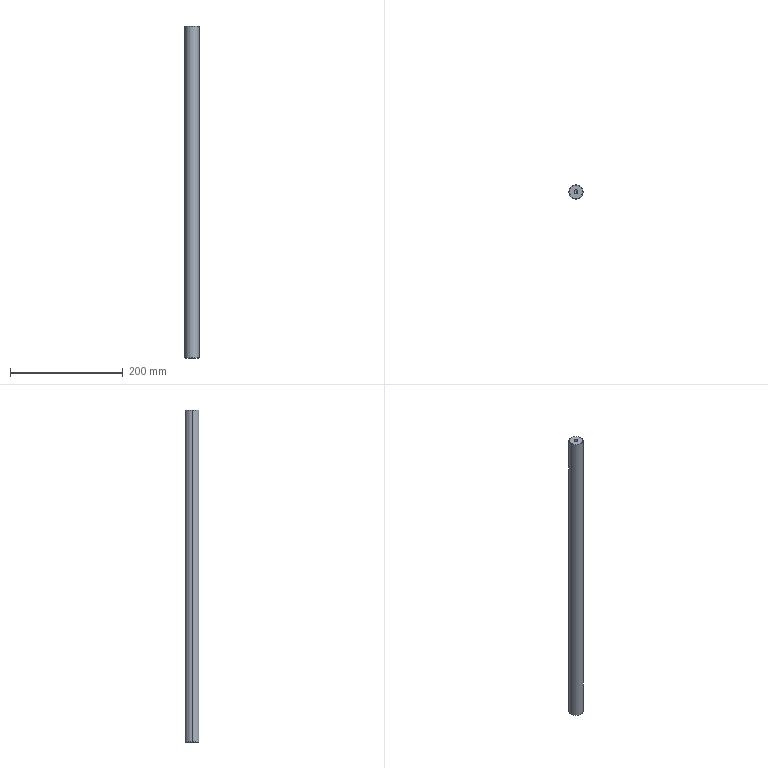Part | SolidWorks | features HoleWzd 2, Chamfer 1, Extrusion 1 | 1 solid | 18 faces | box 25 x 25 x 590 mm | volume 288109 mm3 | cone 10 | cylinder 6 | plane 2 | commonest cylinder face diameters 6.8 x4 25 x2
STEP:
#1=CARTESIAN_POINT('',(12.,0.,590.));
#2=VERTEX_POINT('',#1);
#3=CARTESIAN_POINT('',(-12.,0.,590.));
#4=VERTEX_POINT('',#3);
#5=CARTESIAN_POINT('',(0.,0.,590.));
#6=DIRECTION('',(0.,0.,1.));
#7=DIRECTION('',(1.,0.,0.));
#8=AXIS2_PLACEMENT_3D('',#5,#6,#7);
#9=CIRCLE('',#8,12.);
#10=EDGE_CURVE('',#2,#4,#9,.T.);
#11=ORIENTED_EDGE('',*,*,#10,.F.);
#12=CARTESIAN_POINT('',(12.5,0.,589.5));
#13=VERTEX_POINT('',#12);
#14=CARTESIAN_POINT('',(12.,0.,590.));
#15=DIRECTION('',(0.7071,0.,-0.7071));
#16=VECTOR('',#15,1000.);
#17=LINE('',#14,#16);
#18=EDGE_CURVE('',#2,#13,#17,.T.);
#19=ORIENTED_EDGE('',*,*,#18,.T.);
#20=CARTESIAN_POINT('',(-12.5,0.,589.5));
#21=VERTEX_POINT('',#20);
#22=CARTESIAN_POINT('',(0.,0.,589.5));
#23=DIRECTION('',(0.,0.,-1.));
#24=DIRECTION('',(1.,0.,0.));
#25=AXIS2_PLACEMENT_3D('',#22,#23,#24);
#26=CIRCLE('',#25,12.5);
#27=EDGE_CURVE('',#21,#13,#26,.T.);
#28=ORIENTED_EDGE('',*,*,#27,.F.);
#29=CARTESIAN_POINT('',(-12.,0.,590.));
#30=DIRECTION('',(-0.7071,0.,-0.7071));
#31=VECTOR('',#30,1000.);
#32=LINE('',#29,#31);
#33=EDGE_CURVE('',#4,#21,#32,.T.);
#34=ORIENTED_EDGE('',*,*,#33,.F.);
#35=EDGE_LOOP('',(#11,#19,#28,#34));
#36=FACE_OUTER_BOUND('',#35,.T.);
#37=CARTESIAN_POINT('',(0.,0.,590.));
#38=DIRECTION('',(0.,0.,-1.));
#39=DIRECTION('',(-1.,0.,0.));
#40=AXIS2_PLACEMENT_3D('',#37,#38,#39);
#41=CONICAL_SURFACE('',#40,12.,0.7854);
#42=ADVANCED_FACE('',(#36),#41,.T.);
#43=CARTESIAN_POINT('',(3.4,0.,0.5));
#44=VERTEX_POINT('',#43);
#45=CARTESIAN_POINT('',(-3.4,0.,0.5));
#46=VERTEX_POINT('',#45);
#47=CARTESIAN_POINT('',(0.,0.,0.5));
#48=DIRECTION('',(0.,0.,-1.));
#49=DIRECTION('',(1.,0.,0.));
#50=AXIS2_PLACEMENT_3D('',#47,#48,#49);
#51=CIRCLE('',#50,3.4);
#52=EDGE_CURVE('',#44,#46,#51,.T.);
#53=ORIENTED_EDGE('',*,*,#52,.F.);
#54=CARTESIAN_POINT('',(3.9,0.,0.));
#55=VERTEX_POINT('',#54);
#56=CARTESIAN_POINT('',(3.4,0.,0.5));
#57=DIRECTION('',(0.7071,0.,-0.7071));
#58=VECTOR('',#57,1000.);
#59=LINE('',#56,#58);
#60=EDGE_CURVE('',#44,#55,#59,.T.);
#61=ORIENTED_EDGE('',*,*,#60,.T.);
#62=CARTESIAN_POINT('',(-3.9,0.,0.));
#63=VERTEX_POINT('',#62);
#64=CARTESIAN_POINT('',(0.,0.,0.));
#65=DIRECTION('',(0.,0.,1.));
#66=DIRECTION('',(1.,0.,0.));
#67=AXIS2_PLACEMENT_3D('',#64,#65,#66);
#68=CIRCLE('',#67,3.9);
#69=EDGE_CURVE('',#63,#55,#68,.T.);
#70=ORIENTED_EDGE('',*,*,#69,.F.);
#71=CARTESIAN_POINT('',(-3.4,0.,0.5));
#72=DIRECTION('',(-0.7071,0.,-0.7071));
#73=VECTOR('',#72,1000.);
#74=LINE('',#71,#73);
#75=EDGE_CURVE('',#46,#63,#74,.T.);
#76=ORIENTED_EDGE('',*,*,#75,.F.);
#77=EDGE_LOOP('',(#53,#61,#70,#76));
#78=FACE_OUTER_BOUND('',#77,.T.);
#79=CARTESIAN_POINT('',(0.,0.,0.5));
#80=DIRECTION('',(0.,0.,-1.));
#81=DIRECTION('',(-1.,0.,0.));
#82=AXIS2_PLACEMENT_3D('',#79,#80,#81);
#83=CONICAL_SURFACE('',#82,3.4,0.7854);
#84=ADVANCED_FACE('',(#78),#83,.F.);
#85=CARTESIAN_POINT('',(-12.,0.,0.));
#86=VERTEX_POINT('',#85);
#87=CARTESIAN_POINT('',(12.,0.,0.));
#88=VERTEX_POINT('',#87);
#89=CARTESIAN_POINT('',(0.,0.,0.));
#90=DIRECTION('',(0.,0.,-1.));
#91=DIRECTION('',(1.,0.,0.));
#92=AXIS2_PLACEMENT_3D('',#89,#90,#91);
#93=CIRCLE('',#92,12.);
#94=EDGE_CURVE('',#86,#88,#93,.T.);
#95=ORIENTED_EDGE('',*,*,#94,.F.);
#96=CARTESIAN_POINT('',(-12.5,0.,0.5));
#97=VERTEX_POINT('',#96);
#98=CARTESIAN_POINT('',(-12.5,0.,0.5));
#99=DIRECTION('',(-0.7071,0.,0.7071));
#100=VECTOR('',#99,1000.);
#101=LINE('',#98,#100);
#102=EDGE_CURVE('',#86,#97,#101,.T.);
#103=ORIENTED_EDGE('',*,*,#102,.T.);
#104=CARTESIAN_POINT('',(12.5,0.,0.5));
#105=VERTEX_POINT('',#104);
#106=CARTESIAN_POINT('',(0.,0.,0.5));
#107=DIRECTION('',(0.,0.,1.));
#108=DIRECTION('',(1.,0.,0.));
#109=AXIS2_PLACEMENT_3D('',#106,#107,#108);
#110=CIRCLE('',#109,12.5);
#111=EDGE_CURVE('',#105,#97,#110,.T.);
#112=ORIENTED_EDGE('',*,*,#111,.F.);
#113=CARTESIAN_POINT('',(12.5,0.,0.5));
#114=DIRECTION('',(0.7071,0.,0.7071));
#115=VECTOR('',#114,1000.);
#116=LINE('',#113,#115);
#117=EDGE_CURVE('',#88,#105,#116,.T.);
#118=ORIENTED_EDGE('',*,*,#117,.F.);
#119=EDGE_LOOP('',(#95,#103,#112,#118));
#120=FACE_OUTER_BOUND('',#119,.T.);
#121=CARTESIAN_POINT('',(0.,0.,0.5));
#122=DIRECTION('',(0.,0.,1.));
#123=DIRECTION('',(1.,0.,0.));
#124=AXIS2_PLACEMENT_3D('',#121,#122,#123);
#125=CONICAL_SURFACE('',#124,12.5,0.7854);
#126=ADVANCED_FACE('',(#120),#125,.T.);
#127=CARTESIAN_POINT('',(3.4,0.,19.75));
#128=VERTEX_POINT('',#127);
#129=CARTESIAN_POINT('',(-3.4,0.,19.75));
#130=VERTEX_POINT('',#129);
#131=CARTESIAN_POINT('',(0.,0.,19.75));
#132=DIRECTION('',(0.,0.,-1.));
#133=DIRECTION('',(-1.,0.,0.));
#134=AXIS2_PLACEMENT_3D('',#131,#132,#133);
#135=CIRCLE('',#134,3.4);
#136=EDGE_CURVE('',#128,#130,#135,.T.);
#137=ORIENTED_EDGE('',*,*,#136,.F.);
#138=CARTESIAN_POINT('',(3.4,0.,0.));
#139=DIRECTION('',(0.,0.,-1.));
#140=VECTOR('',#139,1000.);
#141=LINE('',#138,#140);
#142=EDGE_CURVE('',#128,#44,#141,.T.);
#143=ORIENTED_EDGE('',*,*,#142,.T.);
#144=ORIENTED_EDGE('',*,*,#52,.T.);
#145=CARTESIAN_POINT('',(-3.4,0.,0.));
#146=DIRECTION('',(0.,0.,-1.));
#147=VECTOR('',#146,1000.);
#148=LINE('',#145,#147);
#149=EDGE_CURVE('',#130,#46,#148,.T.);
#150=ORIENTED_EDGE('',*,*,#149,.F.);
#151=EDGE_LOOP('',(#137,#143,#144,#150));
#152=FACE_OUTER_BOUND('',#151,.T.);
#153=CARTESIAN_POINT('',(0.,0.,0.));
#154=DIRECTION('',(0.,0.,-1.));
#155=DIRECTION('',(-1.,0.,0.));
#156=AXIS2_PLACEMENT_3D('',#153,#154,#155);
#157=CYLINDRICAL_SURFACE('',#156,3.4);
#158=ADVANCED_FACE('',(#152),#157,.F.);
#159=CARTESIAN_POINT('',(0.,0.,21.793));
#160=VERTEX_POINT('',#159);
#161=CARTESIAN_POINT('',(-3.4,0.,19.75));
#162=DIRECTION('',(-0.8572,0.,-0.515));
#163=VECTOR('',#162,1000.);
#164=LINE('',#161,#163);
#165=EDGE_CURVE('',#160,#130,#164,.T.);
#166=ORIENTED_EDGE('',*,*,#165,.F.);
#167=CARTESIAN_POINT('',(3.4,0.,19.75));
#168=DIRECTION('',(0.8572,0.,-0.515));
#169=VECTOR('',#168,1000.);
#170=LINE('',#167,#169);
#171=EDGE_CURVE('',#160,#128,#170,.T.);
#172=ORIENTED_EDGE('',*,*,#171,.T.);
#173=ORIENTED_EDGE('',*,*,#136,.T.);
#174=EDGE_LOOP('',(#166,#172,#173));
#175=FACE_OUTER_BOUND('',#174,.T.);
#176=CARTESIAN_POINT('',(0.,0.,19.75));
#177=DIRECTION('',(0.,0.,-1.));
#178=DIRECTION('',(-1.,0.,0.));
#179=AXIS2_PLACEMENT_3D('',#176,#177,#178);
#180=CONICAL_SURFACE('',#179,3.4,1.03);
#181=ADVANCED_FACE('',(#175),#180,.F.);
#182=CARTESIAN_POINT('',(-3.4,0.,570.25));
#183=VERTEX_POINT('',#182);
#184=CARTESIAN_POINT('',(3.4,0.,570.25));
#185=VERTEX_POINT('',#184);
#186=CARTESIAN_POINT('',(0.,0.,570.25));
#187=DIRECTION('',(0.,0.,1.));
#188=DIRECTION('',(1.,0.,0.));
#189=AXIS2_PLACEMENT_3D('',#186,#187,#188);
#190=CIRCLE('',#189,3.4);
#191=EDGE_CURVE('',#183,#185,#190,.T.);
#192=ORIENTED_EDGE('',*,*,#191,.F.);
#193=CARTESIAN_POINT('',(-3.4,0.,590.));
#194=VERTEX_POINT('',#193);
#195=CARTESIAN_POINT('',(-3.4,0.,590.));
#196=DIRECTION('',(0.,0.,1.));
#197=VECTOR('',#196,1000.);
#198=LINE('',#195,#197);
#199=EDGE_CURVE('',#183,#194,#198,.T.);
#200=ORIENTED_EDGE('',*,*,#199,.T.);
#201=CARTESIAN_POINT('',(3.4,0.,590.));
#202=VERTEX_POINT('',#201);
#203=CARTESIAN_POINT('',(0.,0.,590.));
#204=DIRECTION('',(0.,0.,1.));
#205=DIRECTION('',(1.,0.,0.));
#206=AXIS2_PLACEMENT_3D('',#203,#204,#205);
#207=CIRCLE('',#206,3.4);
#208=EDGE_CURVE('',#194,#202,#207,.T.);
#209=ORIENTED_EDGE('',*,*,#208,.T.);
#210=CARTESIAN_POINT('',(3.4,0.,590.));
#211=DIRECTION('',(0.,0.,1.));
#212=VECTOR('',#211,1000.);
#213=LINE('',#210,#212);
#214=EDGE_CURVE('',#185,#202,#213,.T.);
#215=ORIENTED_EDGE('',*,*,#214,.F.);
#216=EDGE_LOOP('',(#192,#200,#209,#215));
#217=FACE_OUTER_BOUND('',#216,.T.);
#218=CARTESIAN_POINT('',(0.,0.,590.));
#219=DIRECTION('',(0.,0.,1.));
#220=DIRECTION('',(1.,0.,0.));
#221=AXIS2_PLACEMENT_3D('',#218,#219,#220);
#222=CYLINDRICAL_SURFACE('',#221,3.4);
#223=ADVANCED_FACE('',(#217),#222,.F.);
#224=CARTESIAN_POINT('',(0.,0.,568.207));
#225=VERTEX_POINT('',#224);
#226=CARTESIAN_POINT('',(3.4,0.,570.25));
#227=DIRECTION('',(0.8572,0.,0.515));
#228=VECTOR('',#227,1000.);
#229=LINE('',#226,#228);
#230=EDGE_CURVE('',#225,#185,#229,.T.);
#231=ORIENTED_EDGE('',*,*,#230,.F.);
#232=CARTESIAN_POINT('',(-3.4,0.,570.25));
#233=DIRECTION('',(-0.8572,0.,0.515));
#234=VECTOR('',#233,1000.);
#235=LINE('',#232,#234);
#236=EDGE_CURVE('',#225,#183,#235,.T.);
#237=ORIENTED_EDGE('',*,*,#236,.T.);
#238=ORIENTED_EDGE('',*,*,#191,.T.);
#239=EDGE_LOOP('',(#231,#237,#238));
#240=FACE_OUTER_BOUND('',#239,.T.);
#241=CARTESIAN_POINT('',(0.,0.,570.25));
#242=DIRECTION('',(0.,0.,1.));
#243=DIRECTION('',(1.,0.,0.));
#244=AXIS2_PLACEMENT_3D('',#241,#242,#243);
#245=CONICAL_SURFACE('',#244,3.4,1.03);
#246=ADVANCED_FACE('',(#240),#245,.F.);
#247=ORIENTED_EDGE('',*,*,#27,.T.);
#248=CARTESIAN_POINT('',(12.5,0.,590.));
#249=DIRECTION('',(0.,0.,-1.));
#250=VECTOR('',#249,1000.);
#251=LINE('',#248,#250);
#252=EDGE_CURVE('',#13,#105,#251,.T.);
#253=ORIENTED_EDGE('',*,*,#252,.T.);
#254=ORIENTED_EDGE('',*,*,#111,.T.);
#255=CARTESIAN_POINT('',(-12.5,0.,590.));
#256=DIRECTION('',(0.,0.,-1.));
#257=VECTOR('',#256,1000.);
#258=LINE('',#255,#257);
#259=EDGE_CURVE('',#21,#97,#258,.T.);
#260=ORIENTED_EDGE('',*,*,#259,.F.);
#261=EDGE_LOOP('',(#247,#253,#254,#260));
#262=FACE_OUTER_BOUND('',#261,.T.);
#263=CARTESIAN_POINT('',(0.,0.,590.));
#264=DIRECTION('',(0.,0.,-1.));
#265=DIRECTION('',(-1.,0.,0.));
#266=AXIS2_PLACEMENT_3D('',#263,#264,#265);
#267=CYLINDRICAL_SURFACE('',#266,12.5);
#268=ADVANCED_FACE('',(#262),#267,.T.);
#269=ORIENTED_EDGE('',*,*,#252,.F.);
#270=CARTESIAN_POINT('',(0.,0.,589.5));
#271=DIRECTION('',(0.,0.,-1.));
#272=DIRECTION('',(1.,0.,0.));
#273=AXIS2_PLACEMENT_3D('',#270,#271,#272);
#274=CIRCLE('',#273,12.5);
#275=EDGE_CURVE('',#13,#21,#274,.T.);
#276=ORIENTED_EDGE('',*,*,#275,.T.);
#277=ORIENTED_EDGE('',*,*,#259,.T.);
#278=CARTESIAN_POINT('',(0.,0.,0.5));
#279=DIRECTION('',(0.,0.,1.));
#280=DIRECTION('',(1.,0.,0.));
#281=AXIS2_PLACEMENT_3D('',#278,#279,#280);
#282=CIRCLE('',#281,12.5);
#283=EDGE_CURVE('',#97,#105,#282,.T.);
#284=ORIENTED_EDGE('',*,*,#283,.T.);
#285=EDGE_LOOP('',(#269,#276,#277,#284));
#286=FACE_OUTER_BOUND('',#285,.T.);
#287=CARTESIAN_POINT('',(0.,0.,590.));
#288=DIRECTION('',(0.,0.,-1.));
#289=DIRECTION('',(-1.,0.,0.));
#290=AXIS2_PLACEMENT_3D('',#287,#288,#289);
#291=CYLINDRICAL_SURFACE('',#290,12.5);
#292=ADVANCED_FACE('',(#286),#291,.T.);
#293=CARTESIAN_POINT('',(0.,0.,590.));
#294=DIRECTION('',(0.,0.,1.));
#295=DIRECTION('',(1.,0.,0.));
#296=AXIS2_PLACEMENT_3D('',#293,#294,#295);
#297=CIRCLE('',#296,12.);
#298=EDGE_CURVE('',#4,#2,#297,.T.);
#299=ORIENTED_EDGE('',*,*,#298,.T.);
#300=ORIENTED_EDGE('',*,*,#10,.T.);
#301=EDGE_LOOP('',(#299,#300));
#302=FACE_OUTER_BOUND('',#301,.T.);
#303=CARTESIAN_POINT('',(0.,0.,590.));
#304=DIRECTION('',(0.,0.,1.));
#305=DIRECTION('',(1.,0.,0.));
#306=AXIS2_PLACEMENT_3D('',#303,#304,#305);
#307=CIRCLE('',#306,3.4);
#308=EDGE_CURVE('',#202,#194,#307,.T.);
#309=ORIENTED_EDGE('',*,*,#308,.F.);
#310=ORIENTED_EDGE('',*,*,#208,.F.);
#311=EDGE_LOOP('',(#309,#310));
#312=FACE_BOUND('',#311,.T.);
#313=CARTESIAN_POINT('',(0.,0.,590.));
#314=DIRECTION('',(0.,0.,1.));
#315=DIRECTION('',(1.,0.,0.));
#316=AXIS2_PLACEMENT_3D('',#313,#314,#315);
#317=PLANE('',#316);
#318=ADVANCED_FACE('',(#302,#312),#317,.T.);
#319=CARTESIAN_POINT('',(0.,0.,0.));
#320=DIRECTION('',(0.,0.,-1.));
#321=DIRECTION('',(1.,0.,0.));
#322=AXIS2_PLACEMENT_3D('',#319,#320,#321);
#323=CIRCLE('',#322,12.);
#324=EDGE_CURVE('',#88,#86,#323,.T.);
#325=ORIENTED_EDGE('',*,*,#324,.T.);
#326=ORIENTED_EDGE('',*,*,#94,.T.);
#327=EDGE_LOOP('',(#325,#326));
#328=FACE_OUTER_BOUND('',#327,.T.);
#329=ORIENTED_EDGE('',*,*,#69,.T.);
#330=CARTESIAN_POINT('',(0.,0.,0.));
#331=DIRECTION('',(0.,0.,1.));
#332=DIRECTION('',(1.,0.,0.));
#333=AXIS2_PLACEMENT_3D('',#330,#331,#332);
#334=CIRCLE('',#333,3.9);
#335=EDGE_CURVE('',#55,#63,#334,.T.);
#336=ORIENTED_EDGE('',*,*,#335,.T.);
#337=EDGE_LOOP('',(#329,#336));
#338=FACE_BOUND('',#337,.T.);
#339=CARTESIAN_POINT('',(0.,0.,0.));
#340=DIRECTION('',(0.,0.,1.));
#341=DIRECTION('',(1.,0.,0.));
#342=AXIS2_PLACEMENT_3D('',#339,#340,#341);
#343=PLANE('',#342);
#344=ADVANCED_FACE('',(#328,#338),#343,.F.);
#345=ORIENTED_EDGE('',*,*,#236,.F.);
#346=ORIENTED_EDGE('',*,*,#230,.T.);
#347=CARTESIAN_POINT('',(0.,0.,570.25));
#348=DIRECTION('',(0.,0.,1.));
#349=DIRECTION('',(1.,0.,0.));
#350=AXIS2_PLACEMENT_3D('',#347,#348,#349);
#351=CIRCLE('',#350,3.4);
#352=EDGE_CURVE('',#185,#183,#351,.T.);
#353=ORIENTED_EDGE('',*,*,#352,.T.);
#354=EDGE_LOOP('',(#345,#346,#353));
#355=FACE_OUTER_BOUND('',#354,.T.);
#356=CARTESIAN_POINT('',(0.,0.,570.25));
#357=DIRECTION('',(0.,0.,1.));
#358=DIRECTION('',(1.,0.,0.));
#359=AXIS2_PLACEMENT_3D('',#356,#357,#358);
#360=CONICAL_SURFACE('',#359,3.4,1.03);
#361=ADVANCED_FACE('',(#355),#360,.F.);
#362=ORIENTED_EDGE('',*,*,#199,.F.);
#363=ORIENTED_EDGE('',*,*,#352,.F.);
#364=ORIENTED_EDGE('',*,*,#214,.T.);
#365=ORIENTED_EDGE('',*,*,#308,.T.);
#366=EDGE_LOOP('',(#362,#363,#364,#365));
#367=FACE_OUTER_BOUND('',#366,.T.);
#368=CARTESIAN_POINT('',(0.,0.,590.));
#369=DIRECTION('',(0.,0.,1.));
#370=DIRECTION('',(1.,0.,0.));
#371=AXIS2_PLACEMENT_3D('',#368,#369,#370);
#372=CYLINDRICAL_SURFACE('',#371,3.4);
#373=ADVANCED_FACE('',(#367),#372,.F.);
#374=ORIENTED_EDGE('',*,*,#171,.F.);
#375=ORIENTED_EDGE('',*,*,#165,.T.);
#376=CARTESIAN_POINT('',(0.,0.,19.75));
#377=DIRECTION('',(0.,0.,-1.));
#378=DIRECTION('',(-1.,0.,0.));
#379=AXIS2_PLACEMENT_3D('',#376,#377,#378);
#380=CIRCLE('',#379,3.4);
#381=EDGE_CURVE('',#130,#128,#380,.T.);
#382=ORIENTED_EDGE('',*,*,#381,.T.);
#383=EDGE_LOOP('',(#374,#375,#382));
#384=FACE_OUTER_BOUND('',#383,.T.);
#385=CARTESIAN_POINT('',(0.,0.,19.75));
#386=DIRECTION('',(0.,0.,-1.));
#387=DIRECTION('',(-1.,0.,0.));
#388=AXIS2_PLACEMENT_3D('',#385,#386,#387);
#389=CONICAL_SURFACE('',#388,3.4,1.03);
#390=ADVANCED_FACE('',(#384),#389,.F.);
#391=ORIENTED_EDGE('',*,*,#142,.F.);
#392=ORIENTED_EDGE('',*,*,#381,.F.);
#393=ORIENTED_EDGE('',*,*,#149,.T.);
#394=CARTESIAN_POINT('',(0.,0.,0.5));
#395=DIRECTION('',(0.,0.,-1.));
#396=DIRECTION('',(1.,0.,0.));
#397=AXIS2_PLACEMENT_3D('',#394,#395,#396);
#398=CIRCLE('',#397,3.4);
#399=EDGE_CURVE('',#46,#44,#398,.T.);
#400=ORIENTED_EDGE('',*,*,#399,.T.);
#401=EDGE_LOOP('',(#391,#392,#393,#400));
#402=FACE_OUTER_BOUND('',#401,.T.);
#403=CARTESIAN_POINT('',(0.,0.,0.));
#404=DIRECTION('',(0.,0.,-1.));
#405=DIRECTION('',(-1.,0.,0.));
#406=AXIS2_PLACEMENT_3D('',#403,#404,#405);
#407=CYLINDRICAL_SURFACE('',#406,3.4);
#408=ADVANCED_FACE('',(#402),#407,.F.);
#409=ORIENTED_EDGE('',*,*,#102,.F.);
#410=ORIENTED_EDGE('',*,*,#324,.F.);
#411=ORIENTED_EDGE('',*,*,#117,.T.);
#412=ORIENTED_EDGE('',*,*,#283,.F.);
#413=EDGE_LOOP('',(#409,#410,#411,#412));
#414=FACE_OUTER_BOUND('',#413,.T.);
#415=CARTESIAN_POINT('',(0.,0.,0.5));
#416=DIRECTION('',(0.,0.,1.));
#417=DIRECTION('',(1.,0.,0.));
#418=AXIS2_PLACEMENT_3D('',#415,#416,#417);
#419=CONICAL_SURFACE('',#418,12.5,0.7854);
#420=ADVANCED_FACE('',(#414),#419,.T.);
#421=ORIENTED_EDGE('',*,*,#60,.F.);
#422=ORIENTED_EDGE('',*,*,#399,.F.);
#423=ORIENTED_EDGE('',*,*,#75,.T.);
#424=ORIENTED_EDGE('',*,*,#335,.F.);
#425=EDGE_LOOP('',(#421,#422,#423,#424));
#426=FACE_OUTER_BOUND('',#425,.T.);
#427=CARTESIAN_POINT('',(0.,0.,0.5));
#428=DIRECTION('',(0.,0.,-1.));
#429=DIRECTION('',(-1.,0.,0.));
#430=AXIS2_PLACEMENT_3D('',#427,#428,#429);
#431=CONICAL_SURFACE('',#430,3.4,0.7854);
#432=ADVANCED_FACE('',(#426),#431,.F.);
#433=ORIENTED_EDGE('',*,*,#18,.F.);
#434=ORIENTED_EDGE('',*,*,#298,.F.);
#435=ORIENTED_EDGE('',*,*,#33,.T.);
#436=ORIENTED_EDGE('',*,*,#275,.F.);
#437=EDGE_LOOP('',(#433,#434,#435,#436));
#438=FACE_OUTER_BOUND('',#437,.T.);
#439=CARTESIAN_POINT('',(0.,0.,590.));
#440=DIRECTION('',(0.,0.,-1.));
#441=DIRECTION('',(-1.,0.,0.));
#442=AXIS2_PLACEMENT_3D('',#439,#440,#441);
#443=CONICAL_SURFACE('',#442,12.,0.7854);
#444=ADVANCED_FACE('',(#438),#443,.T.);
#445=CLOSED_SHELL('',(#42,#84,#126,#158,#181,#223,#246,#268,#292,#318,#344,#361,#373,#390,#408,#420,#432,#444));
#446=MANIFOLD_SOLID_BREP('',#445);
#447=CARTESIAN_POINT('',(0.,0.,0.));
#448=DIRECTION('',(0.,0.,1.));
#449=DIRECTION('',(1.,0.,0.));
#450=AXIS2_PLACEMENT_3D('',#447,#448,#449);
#451=(LENGTH_UNIT()NAMED_UNIT(*)SI_UNIT(.MILLI.,.METRE.));
#452=UNCERTAINTY_MEASURE_WITH_UNIT(LENGTH_MEASURE(0.00001),#451,'','');
#453=(NAMED_UNIT(*)PLANE_ANGLE_UNIT()SI_UNIT($,.RADIAN.));
#454=(NAMED_UNIT(*)SI_UNIT($,.STERADIAN.)SOLID_ANGLE_UNIT());
#455=(GEOMETRIC_REPRESENTATION_CONTEXT(3)GLOBAL_UNCERTAINTY_ASSIGNED_CONTEXT((#452))GLOBAL_UNIT_ASSIGNED_CONTEXT((#451,#453,#454))REPRESENTATION_CONTEXT('',''));
#456=ADVANCED_BREP_SHAPE_REPRESENTATION('',(#446,#450),#455);